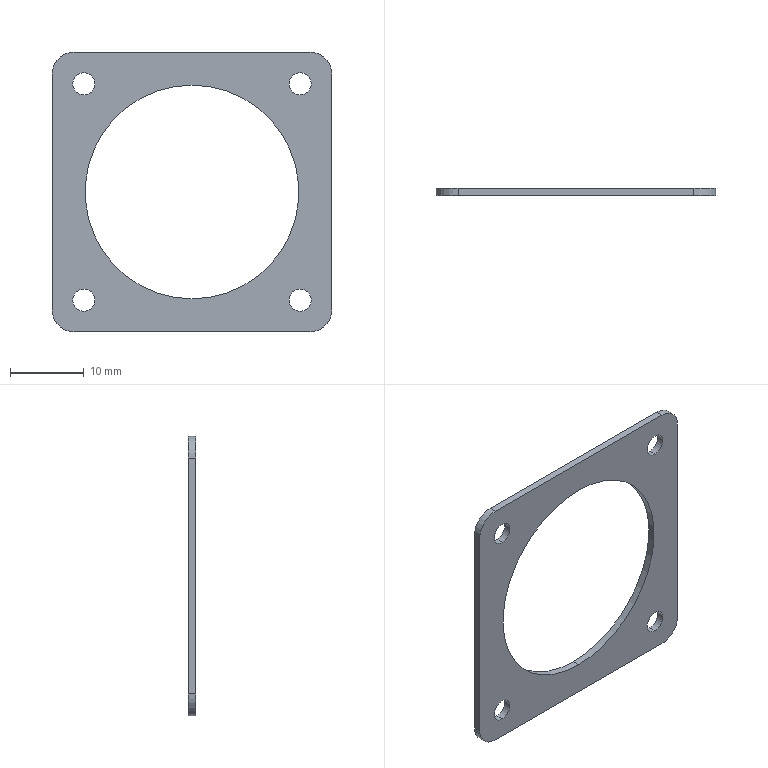Part | STEP file | 15050037_0006 | 1 solid | 20 faces | box 38 x 1 x 38 mm | volume 747.48 mm3 | cylinder 14 | plane 6 | commonest cylinder face diameters 3 x8 6 x4 29 x2